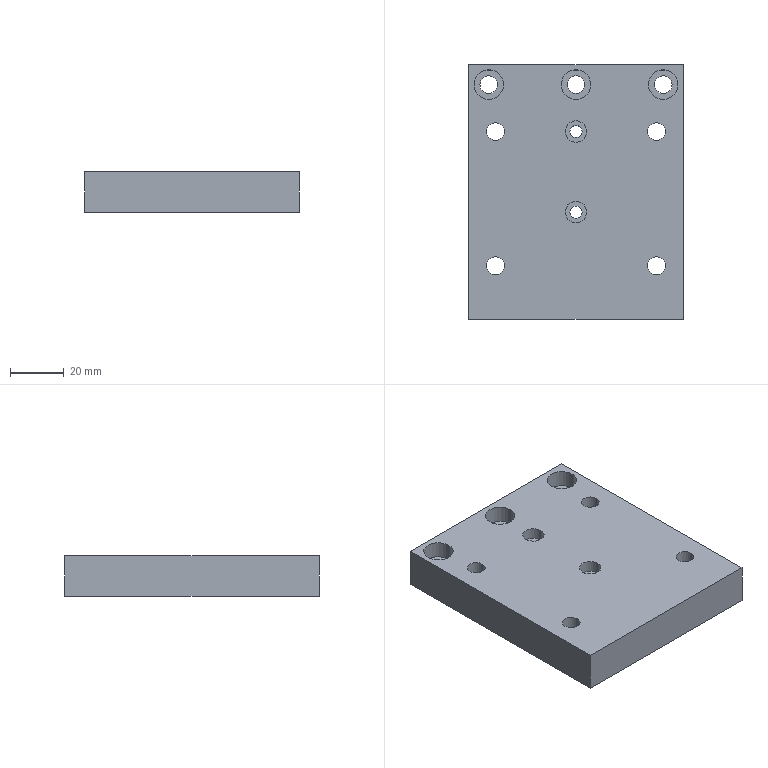Part | SolidWorks | features HoleWzd 3, Extrusion 1 | 1 solid | 51 faces | box 80 x 95 x 15 mm | volume 106903 mm3 | cylinder 36 | plane 15 | commonest cylinder face diameters 6.6 x14 11 x14 4.5 x4 8 x4
STEP:
#1=CARTESIAN_POINT('',(-38.,40.,8.6));
#2=VERTEX_POINT('',#1);
#3=CARTESIAN_POINT('',(-27.,40.,8.6));
#4=VERTEX_POINT('',#3);
#5=CARTESIAN_POINT('',(-32.5,40.,8.6));
#6=DIRECTION('',(0.,0.,1.));
#7=DIRECTION('',(1.,0.,0.));
#8=AXIS2_PLACEMENT_3D('',#5,#6,#7);
#9=CIRCLE('',#8,5.5);
#10=EDGE_CURVE('',#2,#4,#9,.T.);
#11=ORIENTED_EDGE('',*,*,#10,.F.);
#12=CARTESIAN_POINT('',(-38.,40.,15.));
#13=VERTEX_POINT('',#12);
#14=CARTESIAN_POINT('',(-38.,40.,15.));
#15=DIRECTION('',(0.,0.,1.));
#16=VECTOR('',#15,1000.);
#17=LINE('',#14,#16);
#18=EDGE_CURVE('',#2,#13,#17,.T.);
#19=ORIENTED_EDGE('',*,*,#18,.T.);
#20=CARTESIAN_POINT('',(-27.,40.,15.));
#21=VERTEX_POINT('',#20);
#22=CARTESIAN_POINT('',(-32.5,40.,15.));
#23=DIRECTION('',(0.,0.,1.));
#24=DIRECTION('',(1.,0.,0.));
#25=AXIS2_PLACEMENT_3D('',#22,#23,#24);
#26=CIRCLE('',#25,5.5);
#27=EDGE_CURVE('',#13,#21,#26,.T.);
#28=ORIENTED_EDGE('',*,*,#27,.T.);
#29=CARTESIAN_POINT('',(-27.,40.,15.));
#30=DIRECTION('',(0.,0.,1.));
#31=VECTOR('',#30,1000.);
#32=LINE('',#29,#31);
#33=EDGE_CURVE('',#4,#21,#32,.T.);
#34=ORIENTED_EDGE('',*,*,#33,.F.);
#35=EDGE_LOOP('',(#11,#19,#28,#34));
#36=FACE_OUTER_BOUND('',#35,.T.);
#37=CARTESIAN_POINT('',(-32.5,40.,15.));
#38=DIRECTION('',(0.,0.,1.));
#39=DIRECTION('',(1.,0.,0.));
#40=AXIS2_PLACEMENT_3D('',#37,#38,#39);
#41=CYLINDRICAL_SURFACE('',#40,5.5);
#42=ADVANCED_FACE('',(#36),#41,.F.);
#43=CARTESIAN_POINT('',(-35.8,40.,0.));
#44=VERTEX_POINT('',#43);
#45=CARTESIAN_POINT('',(-29.2,40.,0.));
#46=VERTEX_POINT('',#45);
#47=CARTESIAN_POINT('',(-32.5,40.,0.));
#48=DIRECTION('',(0.,0.,1.));
#49=DIRECTION('',(1.,0.,0.));
#50=AXIS2_PLACEMENT_3D('',#47,#48,#49);
#51=CIRCLE('',#50,3.3);
#52=EDGE_CURVE('',#44,#46,#51,.T.);
#53=ORIENTED_EDGE('',*,*,#52,.F.);
#54=CARTESIAN_POINT('',(-35.8,40.,8.6));
#55=VERTEX_POINT('',#54);
#56=CARTESIAN_POINT('',(-35.8,40.,15.));
#57=DIRECTION('',(0.,0.,1.));
#58=VECTOR('',#57,1000.);
#59=LINE('',#56,#58);
#60=EDGE_CURVE('',#44,#55,#59,.T.);
#61=ORIENTED_EDGE('',*,*,#60,.T.);
#62=CARTESIAN_POINT('',(-29.2,40.,8.6));
#63=VERTEX_POINT('',#62);
#64=CARTESIAN_POINT('',(-32.5,40.,8.6));
#65=DIRECTION('',(0.,0.,1.));
#66=DIRECTION('',(1.,0.,0.));
#67=AXIS2_PLACEMENT_3D('',#64,#65,#66);
#68=CIRCLE('',#67,3.3);
#69=EDGE_CURVE('',#55,#63,#68,.T.);
#70=ORIENTED_EDGE('',*,*,#69,.T.);
#71=CARTESIAN_POINT('',(-29.2,40.,15.));
#72=DIRECTION('',(0.,0.,1.));
#73=VECTOR('',#72,1000.);
#74=LINE('',#71,#73);
#75=EDGE_CURVE('',#46,#63,#74,.T.);
#76=ORIENTED_EDGE('',*,*,#75,.F.);
#77=EDGE_LOOP('',(#53,#61,#70,#76));
#78=FACE_OUTER_BOUND('',#77,.T.);
#79=CARTESIAN_POINT('',(-32.5,40.,15.));
#80=DIRECTION('',(0.,0.,1.));
#81=DIRECTION('',(1.,0.,0.));
#82=AXIS2_PLACEMENT_3D('',#79,#80,#81);
#83=CYLINDRICAL_SURFACE('',#82,3.3);
#84=ADVANCED_FACE('',(#78),#83,.F.);
#85=CARTESIAN_POINT('',(-5.5,40.,8.6));
#86=VERTEX_POINT('',#85);
#87=CARTESIAN_POINT('',(5.5,40.,8.6));
#88=VERTEX_POINT('',#87);
#89=CARTESIAN_POINT('',(0.,40.,8.6));
#90=DIRECTION('',(0.,0.,1.));
#91=DIRECTION('',(1.,0.,0.));
#92=AXIS2_PLACEMENT_3D('',#89,#90,#91);
#93=CIRCLE('',#92,5.5);
#94=EDGE_CURVE('',#86,#88,#93,.T.);
#95=ORIENTED_EDGE('',*,*,#94,.F.);
#96=CARTESIAN_POINT('',(-5.5,40.,15.));
#97=VERTEX_POINT('',#96);
#98=CARTESIAN_POINT('',(-5.5,40.,15.));
#99=DIRECTION('',(0.,0.,1.));
#100=VECTOR('',#99,1000.);
#101=LINE('',#98,#100);
#102=EDGE_CURVE('',#86,#97,#101,.T.);
#103=ORIENTED_EDGE('',*,*,#102,.T.);
#104=CARTESIAN_POINT('',(5.5,40.,15.));
#105=VERTEX_POINT('',#104);
#106=CARTESIAN_POINT('',(0.,40.,15.));
#107=DIRECTION('',(0.,0.,1.));
#108=DIRECTION('',(1.,0.,0.));
#109=AXIS2_PLACEMENT_3D('',#106,#107,#108);
#110=CIRCLE('',#109,5.5);
#111=EDGE_CURVE('',#97,#105,#110,.T.);
#112=ORIENTED_EDGE('',*,*,#111,.T.);
#113=CARTESIAN_POINT('',(5.5,40.,15.));
#114=DIRECTION('',(0.,0.,1.));
#115=VECTOR('',#114,1000.);
#116=LINE('',#113,#115);
#117=EDGE_CURVE('',#88,#105,#116,.T.);
#118=ORIENTED_EDGE('',*,*,#117,.F.);
#119=EDGE_LOOP('',(#95,#103,#112,#118));
#120=FACE_OUTER_BOUND('',#119,.T.);
#121=CARTESIAN_POINT('',(0.,40.,15.));
#122=DIRECTION('',(0.,0.,1.));
#123=DIRECTION('',(1.,0.,0.));
#124=AXIS2_PLACEMENT_3D('',#121,#122,#123);
#125=CYLINDRICAL_SURFACE('',#124,5.5);
#126=ADVANCED_FACE('',(#120),#125,.F.);
#127=CARTESIAN_POINT('',(-3.3,40.,0.));
#128=VERTEX_POINT('',#127);
#129=CARTESIAN_POINT('',(3.3,40.,0.));
#130=VERTEX_POINT('',#129);
#131=CARTESIAN_POINT('',(0.,40.,0.));
#132=DIRECTION('',(0.,0.,1.));
#133=DIRECTION('',(1.,0.,0.));
#134=AXIS2_PLACEMENT_3D('',#131,#132,#133);
#135=CIRCLE('',#134,3.3);
#136=EDGE_CURVE('',#128,#130,#135,.T.);
#137=ORIENTED_EDGE('',*,*,#136,.F.);
#138=CARTESIAN_POINT('',(-3.3,40.,8.6));
#139=VERTEX_POINT('',#138);
#140=CARTESIAN_POINT('',(-3.3,40.,15.));
#141=DIRECTION('',(0.,0.,1.));
#142=VECTOR('',#141,1000.);
#143=LINE('',#140,#142);
#144=EDGE_CURVE('',#128,#139,#143,.T.);
#145=ORIENTED_EDGE('',*,*,#144,.T.);
#146=CARTESIAN_POINT('',(3.3,40.,8.6));
#147=VERTEX_POINT('',#146);
#148=CARTESIAN_POINT('',(0.,40.,8.6));
#149=DIRECTION('',(0.,0.,1.));
#150=DIRECTION('',(1.,0.,0.));
#151=AXIS2_PLACEMENT_3D('',#148,#149,#150);
#152=CIRCLE('',#151,3.3);
#153=EDGE_CURVE('',#139,#147,#152,.T.);
#154=ORIENTED_EDGE('',*,*,#153,.T.);
#155=CARTESIAN_POINT('',(3.3,40.,15.));
#156=DIRECTION('',(0.,0.,1.));
#157=VECTOR('',#156,1000.);
#158=LINE('',#155,#157);
#159=EDGE_CURVE('',#130,#147,#158,.T.);
#160=ORIENTED_EDGE('',*,*,#159,.F.);
#161=EDGE_LOOP('',(#137,#145,#154,#160));
#162=FACE_OUTER_BOUND('',#161,.T.);
#163=CARTESIAN_POINT('',(0.,40.,15.));
#164=DIRECTION('',(0.,0.,1.));
#165=DIRECTION('',(1.,0.,0.));
#166=AXIS2_PLACEMENT_3D('',#163,#164,#165);
#167=CYLINDRICAL_SURFACE('',#166,3.3);
#168=ADVANCED_FACE('',(#162),#167,.F.);
#169=CARTESIAN_POINT('',(27.,40.,8.6));
#170=VERTEX_POINT('',#169);
#171=CARTESIAN_POINT('',(38.,40.,8.6));
#172=VERTEX_POINT('',#171);
#173=CARTESIAN_POINT('',(32.5,40.,8.6));
#174=DIRECTION('',(0.,0.,1.));
#175=DIRECTION('',(1.,0.,0.));
#176=AXIS2_PLACEMENT_3D('',#173,#174,#175);
#177=CIRCLE('',#176,5.5);
#178=EDGE_CURVE('',#170,#172,#177,.T.);
#179=ORIENTED_EDGE('',*,*,#178,.F.);
#180=CARTESIAN_POINT('',(27.,40.,15.));
#181=VERTEX_POINT('',#180);
#182=CARTESIAN_POINT('',(27.,40.,15.));
#183=DIRECTION('',(0.,0.,1.));
#184=VECTOR('',#183,1000.);
#185=LINE('',#182,#184);
#186=EDGE_CURVE('',#170,#181,#185,.T.);
#187=ORIENTED_EDGE('',*,*,#186,.T.);
#188=CARTESIAN_POINT('',(38.,40.,15.));
#189=VERTEX_POINT('',#188);
#190=CARTESIAN_POINT('',(32.5,40.,15.));
#191=DIRECTION('',(0.,0.,1.));
#192=DIRECTION('',(1.,0.,0.));
#193=AXIS2_PLACEMENT_3D('',#190,#191,#192);
#194=CIRCLE('',#193,5.5);
#195=EDGE_CURVE('',#181,#189,#194,.T.);
#196=ORIENTED_EDGE('',*,*,#195,.T.);
#197=CARTESIAN_POINT('',(38.,40.,15.));
#198=DIRECTION('',(0.,0.,1.));
#199=VECTOR('',#198,1000.);
#200=LINE('',#197,#199);
#201=EDGE_CURVE('',#172,#189,#200,.T.);
#202=ORIENTED_EDGE('',*,*,#201,.F.);
#203=EDGE_LOOP('',(#179,#187,#196,#202));
#204=FACE_OUTER_BOUND('',#203,.T.);
#205=CARTESIAN_POINT('',(32.5,40.,15.));
#206=DIRECTION('',(0.,0.,1.));
#207=DIRECTION('',(1.,0.,0.));
#208=AXIS2_PLACEMENT_3D('',#205,#206,#207);
#209=CYLINDRICAL_SURFACE('',#208,5.5);
#210=ADVANCED_FACE('',(#204),#209,.F.);
#211=CARTESIAN_POINT('',(29.2,40.,0.));
#212=VERTEX_POINT('',#211);
#213=CARTESIAN_POINT('',(35.8,40.,0.));
#214=VERTEX_POINT('',#213);
#215=CARTESIAN_POINT('',(32.5,40.,0.));
#216=DIRECTION('',(0.,0.,1.));
#217=DIRECTION('',(1.,0.,0.));
#218=AXIS2_PLACEMENT_3D('',#215,#216,#217);
#219=CIRCLE('',#218,3.3);
#220=EDGE_CURVE('',#212,#214,#219,.T.);
#221=ORIENTED_EDGE('',*,*,#220,.F.);
#222=CARTESIAN_POINT('',(29.2,40.,8.6));
#223=VERTEX_POINT('',#222);
#224=CARTESIAN_POINT('',(29.2,40.,15.));
#225=DIRECTION('',(0.,0.,1.));
#226=VECTOR('',#225,1000.);
#227=LINE('',#224,#226);
#228=EDGE_CURVE('',#212,#223,#227,.T.);
#229=ORIENTED_EDGE('',*,*,#228,.T.);
#230=CARTESIAN_POINT('',(35.8,40.,8.6));
#231=VERTEX_POINT('',#230);
#232=CARTESIAN_POINT('',(32.5,40.,8.6));
#233=DIRECTION('',(0.,0.,1.));
#234=DIRECTION('',(1.,0.,0.));
#235=AXIS2_PLACEMENT_3D('',#232,#233,#234);
#236=CIRCLE('',#235,3.3);
#237=EDGE_CURVE('',#223,#231,#236,.T.);
#238=ORIENTED_EDGE('',*,*,#237,.T.);
#239=CARTESIAN_POINT('',(35.8,40.,15.));
#240=DIRECTION('',(0.,0.,1.));
#241=VECTOR('',#240,1000.);
#242=LINE('',#239,#241);
#243=EDGE_CURVE('',#214,#231,#242,.T.);
#244=ORIENTED_EDGE('',*,*,#243,.F.);
#245=EDGE_LOOP('',(#221,#229,#238,#244));
#246=FACE_OUTER_BOUND('',#245,.T.);
#247=CARTESIAN_POINT('',(32.5,40.,15.));
#248=DIRECTION('',(0.,0.,1.));
#249=DIRECTION('',(1.,0.,0.));
#250=AXIS2_PLACEMENT_3D('',#247,#248,#249);
#251=CYLINDRICAL_SURFACE('',#250,3.3);
#252=ADVANCED_FACE('',(#246),#251,.F.);
#253=CARTESIAN_POINT('',(35.5,22.5,6.4));
#254=VERTEX_POINT('',#253);
#255=CARTESIAN_POINT('',(24.5,22.5,6.4));
#256=VERTEX_POINT('',#255);
#257=CARTESIAN_POINT('',(30.,22.5,6.4));
#258=DIRECTION('',(0.,0.,-1.));
#259=DIRECTION('',(-1.,0.,0.));
#260=AXIS2_PLACEMENT_3D('',#257,#258,#259);
#261=CIRCLE('',#260,5.5);
#262=EDGE_CURVE('',#254,#256,#261,.T.);
#263=ORIENTED_EDGE('',*,*,#262,.F.);
#264=CARTESIAN_POINT('',(35.5,22.5,0.));
#265=VERTEX_POINT('',#264);
#266=CARTESIAN_POINT('',(35.5,22.5,0.));
#267=DIRECTION('',(0.,0.,-1.));
#268=VECTOR('',#267,1000.);
#269=LINE('',#266,#268);
#270=EDGE_CURVE('',#254,#265,#269,.T.);
#271=ORIENTED_EDGE('',*,*,#270,.T.);
#272=CARTESIAN_POINT('',(24.5,22.5,0.));
#273=VERTEX_POINT('',#272);
#274=CARTESIAN_POINT('',(30.,22.5,0.));
#275=DIRECTION('',(0.,0.,-1.));
#276=DIRECTION('',(-1.,0.,0.));
#277=AXIS2_PLACEMENT_3D('',#274,#275,#276);
#278=CIRCLE('',#277,5.5);
#279=EDGE_CURVE('',#265,#273,#278,.T.);
#280=ORIENTED_EDGE('',*,*,#279,.T.);
#281=CARTESIAN_POINT('',(24.5,22.5,0.));
#282=DIRECTION('',(0.,0.,-1.));
#283=VECTOR('',#282,1000.);
#284=LINE('',#281,#283);
#285=EDGE_CURVE('',#256,#273,#284,.T.);
#286=ORIENTED_EDGE('',*,*,#285,.F.);
#287=EDGE_LOOP('',(#263,#271,#280,#286));
#288=FACE_OUTER_BOUND('',#287,.T.);
#289=CARTESIAN_POINT('',(30.,22.5,0.));
#290=DIRECTION('',(0.,0.,-1.));
#291=DIRECTION('',(-1.,0.,0.));
#292=AXIS2_PLACEMENT_3D('',#289,#290,#291);
#293=CYLINDRICAL_SURFACE('',#292,5.5);
#294=ADVANCED_FACE('',(#288),#293,.F.);
#295=CARTESIAN_POINT('',(33.3,22.5,15.));
#296=VERTEX_POINT('',#295);
#297=CARTESIAN_POINT('',(26.7,22.5,15.));
#298=VERTEX_POINT('',#297);
#299=CARTESIAN_POINT('',(30.,22.5,15.));
#300=DIRECTION('',(0.,0.,-1.));
#301=DIRECTION('',(-1.,0.,0.));
#302=AXIS2_PLACEMENT_3D('',#299,#300,#301);
#303=CIRCLE('',#302,3.3);
#304=EDGE_CURVE('',#296,#298,#303,.T.);
#305=ORIENTED_EDGE('',*,*,#304,.F.);
#306=CARTESIAN_POINT('',(33.3,22.5,6.4));
#307=VERTEX_POINT('',#306);
#308=CARTESIAN_POINT('',(33.3,22.5,0.));
#309=DIRECTION('',(0.,0.,-1.));
#310=VECTOR('',#309,1000.);
#311=LINE('',#308,#310);
#312=EDGE_CURVE('',#296,#307,#311,.T.);
#313=ORIENTED_EDGE('',*,*,#312,.T.);
#314=CARTESIAN_POINT('',(26.7,22.5,6.4));
#315=VERTEX_POINT('',#314);
#316=CARTESIAN_POINT('',(30.,22.5,6.4));
#317=DIRECTION('',(0.,0.,-1.));
#318=DIRECTION('',(-1.,0.,0.));
#319=AXIS2_PLACEMENT_3D('',#316,#317,#318);
#320=CIRCLE('',#319,3.3);
#321=EDGE_CURVE('',#307,#315,#320,.T.);
#322=ORIENTED_EDGE('',*,*,#321,.T.);
#323=CARTESIAN_POINT('',(26.7,22.5,0.));
#324=DIRECTION('',(0.,0.,-1.));
#325=VECTOR('',#324,1000.);
#326=LINE('',#323,#325);
#327=EDGE_CURVE('',#298,#315,#326,.T.);
#328=ORIENTED_EDGE('',*,*,#327,.F.);
#329=EDGE_LOOP('',(#305,#313,#322,#328));
#330=FACE_OUTER_BOUND('',#329,.T.);
#331=CARTESIAN_POINT('',(30.,22.5,0.));
#332=DIRECTION('',(0.,0.,-1.));
#333=DIRECTION('',(-1.,0.,0.));
#334=AXIS2_PLACEMENT_3D('',#331,#332,#333);
#335=CYLINDRICAL_SURFACE('',#334,3.3);
#336=ADVANCED_FACE('',(#330),#335,.F.);
#337=CARTESIAN_POINT('',(-24.5,22.5,6.4));
#338=VERTEX_POINT('',#337);
#339=CARTESIAN_POINT('',(-35.5,22.5,6.4));
#340=VERTEX_POINT('',#339);
#341=CARTESIAN_POINT('',(-30.,22.5,6.4));
#342=DIRECTION('',(0.,0.,-1.));
#343=DIRECTION('',(-1.,0.,0.));
#344=AXIS2_PLACEMENT_3D('',#341,#342,#343);
#345=CIRCLE('',#344,5.5);
#346=EDGE_CURVE('',#338,#340,#345,.T.);
#347=ORIENTED_EDGE('',*,*,#346,.F.);
#348=CARTESIAN_POINT('',(-24.5,22.5,0.));
#349=VERTEX_POINT('',#348);
#350=CARTESIAN_POINT('',(-24.5,22.5,0.));
#351=DIRECTION('',(0.,0.,-1.));
#352=VECTOR('',#351,1000.);
#353=LINE('',#350,#352);
#354=EDGE_CURVE('',#338,#349,#353,.T.);
#355=ORIENTED_EDGE('',*,*,#354,.T.);
#356=CARTESIAN_POINT('',(-35.5,22.5,0.));
#357=VERTEX_POINT('',#356);
#358=CARTESIAN_POINT('',(-30.,22.5,0.));
#359=DIRECTION('',(0.,0.,-1.));
#360=DIRECTION('',(-1.,0.,0.));
#361=AXIS2_PLACEMENT_3D('',#358,#359,#360);
#362=CIRCLE('',#361,5.5);
#363=EDGE_CURVE('',#349,#357,#362,.T.);
#364=ORIENTED_EDGE('',*,*,#363,.T.);
#365=CARTESIAN_POINT('',(-35.5,22.5,0.));
#366=DIRECTION('',(0.,0.,-1.));
#367=VECTOR('',#366,1000.);
#368=LINE('',#365,#367);
#369=EDGE_CURVE('',#340,#357,#368,.T.);
#370=ORIENTED_EDGE('',*,*,#369,.F.);
#371=EDGE_LOOP('',(#347,#355,#364,#370));
#372=FACE_OUTER_BOUND('',#371,.T.);
#373=CARTESIAN_POINT('',(-30.,22.5,0.));
#374=DIRECTION('',(0.,0.,-1.));
#375=DIRECTION('',(-1.,0.,0.));
#376=AXIS2_PLACEMENT_3D('',#373,#374,#375);
#377=CYLINDRICAL_SURFACE('',#376,5.5);
#378=ADVANCED_FACE('',(#372),#377,.F.);
#379=CARTESIAN_POINT('',(-26.7,22.5,15.));
#380=VERTEX_POINT('',#379);
#381=CARTESIAN_POINT('',(-33.3,22.5,15.));
#382=VERTEX_POINT('',#381);
#383=CARTESIAN_POINT('',(-30.,22.5,15.));
#384=DIRECTION('',(0.,0.,-1.));
#385=DIRECTION('',(-1.,0.,0.));
#386=AXIS2_PLACEMENT_3D('',#383,#384,#385);
#387=CIRCLE('',#386,3.3);
#388=EDGE_CURVE('',#380,#382,#387,.T.);
#389=ORIENTED_EDGE('',*,*,#388,.F.);
#390=CARTESIAN_POINT('',(-26.7,22.5,6.4));
#391=VERTEX_POINT('',#390);
#392=CARTESIAN_POINT('',(-26.7,22.5,0.));
#393=DIRECTION('',(0.,0.,-1.));
#394=VECTOR('',#393,1000.);
#395=LINE('',#392,#394);
#396=EDGE_CURVE('',#380,#391,#395,.T.);
#397=ORIENTED_EDGE('',*,*,#396,.T.);
#398=CARTESIAN_POINT('',(-33.3,22.5,6.4));
#399=VERTEX_POINT('',#398);
#400=CARTESIAN_POINT('',(-30.,22.5,6.4));
#401=DIRECTION('',(0.,0.,-1.));
#402=DIRECTION('',(-1.,0.,0.));
#403=AXIS2_PLACEMENT_3D('',#400,#401,#402);
#404=CIRCLE('',#403,3.3);
#405=EDGE_CURVE('',#391,#399,#404,.T.);
#406=ORIENTED_EDGE('',*,*,#405,.T.);
#407=CARTESIAN_POINT('',(-33.3,22.5,0.));
#408=DIRECTION('',(0.,0.,-1.));
#409=VECTOR('',#408,1000.);
#410=LINE('',#407,#409);
#411=EDGE_CURVE('',#382,#399,#410,.T.);
#412=ORIENTED_EDGE('',*,*,#411,.F.);
#413=EDGE_LOOP('',(#389,#397,#406,#412));
#414=FACE_OUTER_BOUND('',#413,.T.);
#415=CARTESIAN_POINT('',(-30.,22.5,0.));
#416=DIRECTION('',(0.,0.,-1.));
#417=DIRECTION('',(-1.,0.,0.));
#418=AXIS2_PLACEMENT_3D('',#415,#416,#417);
#419=CYLINDRICAL_SURFACE('',#418,3.3);
#420=ADVANCED_FACE('',(#414),#419,.F.);
#421=CARTESIAN_POINT('',(-24.5,-27.5,6.4));
#422=VERTEX_POINT('',#421);
#423=CARTESIAN_POINT('',(-35.5,-27.5,6.4));
#424=VERTEX_POINT('',#423);
#425=CARTESIAN_POINT('',(-30.,-27.5,6.4));
#426=DIRECTION('',(0.,0.,-1.));
#427=DIRECTION('',(-1.,0.,0.));
#428=AXIS2_PLACEMENT_3D('',#425,#426,#427);
#429=CIRCLE('',#428,5.5);
#430=EDGE_CURVE('',#422,#424,#429,.T.);
#431=ORIENTED_EDGE('',*,*,#430,.F.);
#432=CARTESIAN_POINT('',(-24.5,-27.5,0.));
#433=VERTEX_POINT('',#432);
#434=CARTESIAN_POINT('',(-24.5,-27.5,0.));
#435=DIRECTION('',(0.,0.,-1.));
#436=VECTOR('',#435,1000.);
#437=LINE('',#434,#436);
#438=EDGE_CURVE('',#422,#433,#437,.T.);
#439=ORIENTED_EDGE('',*,*,#438,.T.);
#440=CARTESIAN_POINT('',(-35.5,-27.5,0.));
#441=VERTEX_POINT('',#440);
#442=CARTESIAN_POINT('',(-30.,-27.5,0.));
#443=DIRECTION('',(0.,0.,-1.));
#444=DIRECTION('',(-1.,0.,0.));
#445=AXIS2_PLACEMENT_3D('',#442,#443,#444);
#446=CIRCLE('',#445,5.5);
#447=EDGE_CURVE('',#433,#441,#446,.T.);
#448=ORIENTED_EDGE('',*,*,#447,.T.);
#449=CARTESIAN_POINT('',(-35.5,-27.5,0.));
#450=DIRECTION('',(0.,0.,-1.));
#451=VECTOR('',#450,1000.);
#452=LINE('',#449,#451);
#453=EDGE_CURVE('',#424,#441,#452,.T.);
#454=ORIENTED_EDGE('',*,*,#453,.F.);
#455=EDGE_LOOP('',(#431,#439,#448,#454));
#456=FACE_OUTER_BOUND('',#455,.T.);
#457=CARTESIAN_POINT('',(-30.,-27.5,0.));
#458=DIRECTION('',(0.,0.,-1.));
#459=DIRECTION('',(-1.,0.,0.));
#460=AXIS2_PLACEMENT_3D('',#457,#458,#459);
#461=CYLINDRICAL_SURFACE('',#460,5.5);
#462=ADVANCED_FACE('',(#456),#461,.F.);
#463=CARTESIAN_POINT('',(-26.7,-27.5,15.));
#464=VERTEX_POINT('',#463);
#465=CARTESIAN_POINT('',(-33.3,-27.5,15.));
#466=VERTEX_POINT('',#465);
#467=CARTESIAN_POINT('',(-30.,-27.5,15.));
#468=DIRECTION('',(0.,0.,-1.));
#469=DIRECTION('',(-1.,0.,0.));
#470=AXIS2_PLACEMENT_3D('',#467,#468,#469);
#471=CIRCLE('',#470,3.3);
#472=EDGE_CURVE('',#464,#466,#471,.T.);
#473=ORIENTED_EDGE('',*,*,#472,.F.);
#474=CARTESIAN_POINT('',(-26.7,-27.5,6.4));
#475=VERTEX_POINT('',#474);
#476=CARTESIAN_POINT('',(-26.7,-27.5,0.));
#477=DIRECTION('',(0.,0.,-1.));
#478=VECTOR('',#477,1000.);
#479=LINE('',#476,#478);
#480=EDGE_CURVE('',#464,#475,#479,.T.);
#481=ORIENTED_EDGE('',*,*,#480,.T.);
#482=CARTESIAN_POINT('',(-33.3,-27.5,6.4));
#483=VERTEX_POINT('',#482);
#484=CARTESIAN_POINT('',(-30.,-27.5,6.4));
#485=DIRECTION('',(0.,0.,-1.));
#486=DIRECTION('',(-1.,0.,0.));
#487=AXIS2_PLACEMENT_3D('',#484,#485,#486);
#488=CIRCLE('',#487,3.3);
#489=EDGE_CURVE('',#475,#483,#488,.T.);
#490=ORIENTED_EDGE('',*,*,#489,.T.);
#491=CARTESIAN_POINT('',(-33.3,-27.5,0.));
#492=DIRECTION('',(0.,0.,-1.));
#493=VECTOR('',#492,1000.);
#494=LINE('',#491,#493);
#495=EDGE_CURVE('',#466,#483,#494,.T.);
#496=ORIENTED_EDGE('',*,*,#495,.F.);
#497=EDGE_LOOP('',(#473,#481,#490,#496));
#498=FACE_OUTER_BOUND('',#497,.T.);
#499=CARTESIAN_POINT('',(-30.,-27.5,0.));
#500=DIRECTION('',(0.,0.,-1.));
#501=DIRECTION('',(-1.,0.,0.));
#502=AXIS2_PLACEMENT_3D('',#499,#500,#501);
#503=CYLINDRICAL_SURFACE('',#502,3.3);
#504=ADVANCED_FACE('',(#498),#503,.F.);
#505=CARTESIAN_POINT('',(35.5,-27.5,6.4));
#506=VERTEX_POINT('',#505);
#507=CARTESIAN_POINT('',(24.5,-27.5,6.4));
#508=VERTEX_POINT('',#507);
#509=CARTESIAN_POINT('',(30.,-27.5,6.4));
#510=DIRECTION('',(0.,0.,-1.));
#511=DIRECTION('',(-1.,0.,0.));
#512=AXIS2_PLACEMENT_3D('',#509,#510,#511);
#513=CIRCLE('',#512,5.5);
#514=EDGE_CURVE('',#506,#508,#513,.T.);
#515=ORIENTED_EDGE('',*,*,#514,.F.);
#516=CARTESIAN_POINT('',(35.5,-27.5,0.));
#517=VERTEX_POINT('',#516);
#518=CARTESIAN_POINT('',(35.5,-27.5,0.));
#519=DIRECTION('',(0.,0.,-1.));
#520=VECTOR('',#519,1000.);
#521=LINE('',#518,#520);
#522=EDGE_CURVE('',#506,#517,#521,.T.);
#523=ORIENTED_EDGE('',*,*,#522,.T.);
#524=CARTESIAN_POINT('',(24.5,-27.5,0.));
#525=VERTEX_POINT('',#524);
#526=CARTESIAN_POINT('',(30.,-27.5,0.));
#527=DIRECTION('',(0.,0.,-1.));
#528=DIRECTION('',(-1.,0.,0.));
#529=AXIS2_PLACEMENT_3D('',#526,#527,#528);
#530=CIRCLE('',#529,5.5);
#531=EDGE_CURVE('',#517,#525,#530,.T.);
#532=ORIENTED_EDGE('',*,*,#531,.T.);
#533=CARTESIAN_POINT('',(24.5,-27.5,0.));
#534=DIRECTION('',(0.,0.,-1.));
#535=VECTOR('',#534,1000.);
#536=LINE('',#533,#535);
#537=EDGE_CURVE('',#508,#525,#536,.T.);
#538=ORIENTED_EDGE('',*,*,#537,.F.);
#539=EDGE_LOOP('',(#515,#523,#532,#538));
#540=FACE_OUTER_BOUND('',#539,.T.);
#541=CARTESIAN_POINT('',(30.,-27.5,0.));
#542=DIRECTION('',(0.,0.,-1.));
#543=DIRECTION('',(-1.,0.,0.));
#544=AXIS2_PLACEMENT_3D('',#541,#542,#543);
#545=CYLINDRICAL_SURFACE('',#544,5.5);
#546=ADVANCED_FACE('',(#540),#545,.F.);
#547=CARTESIAN_POINT('',(33.3,-27.5,15.));
#548=VERTEX_POINT('',#547);
#549=CARTESIAN_POINT('',(26.7,-27.5,15.));
#550=VERTEX_POINT('',#549);
#551=CARTESIAN_POINT('',(30.,-27.5,15.));
#552=DIRECTION('',(0.,0.,-1.));
#553=DIRECTION('',(-1.,0.,0.));
#554=AXIS2_PLACEMENT_3D('',#551,#552,#553);
#555=CIRCLE('',#554,3.3);
#556=EDGE_CURVE('',#548,#550,#555,.T.);
#557=ORIENTED_EDGE('',*,*,#556,.F.);
#558=CARTESIAN_POINT('',(33.3,-27.5,6.4));
#559=VERTEX_POINT('',#558);
#560=CARTESIAN_POINT('',(33.3,-27.5,0.));
#561=DIRECTION('',(0.,0.,-1.));
#562=VECTOR('',#561,1000.);
#563=LINE('',#560,#562);
#564=EDGE_CURVE('',#548,#559,#563,.T.);
#565=ORIENTED_EDGE('',*,*,#564,.T.);
#566=CARTESIAN_POINT('',(26.7,-27.5,6.4));
#567=VERTEX_POINT('',#566);
#568=CARTESIAN_POINT('',(30.,-27.5,6.4));
#569=DIRECTION('',(0.,0.,-1.));
#570=DIRECTION('',(-1.,0.,0.));
#571=AXIS2_PLACEMENT_3D('',#568,#569,#570);
#572=CIRCLE('',#571,3.3);
#573=EDGE_CURVE('',#559,#567,#572,.T.);
#574=ORIENTED_EDGE('',*,*,#573,.T.);
#575=CARTESIAN_POINT('',(26.7,-27.5,0.));
#576=DIRECTION('',(0.,0.,-1.));
#577=VECTOR('',#576,1000.);
#578=LINE('',#575,#577);
#579=EDGE_CURVE('',#550,#567,#578,.T.);
#580=ORIENTED_EDGE('',*,*,#579,.F.);
#581=EDGE_LOOP('',(#557,#565,#574,#580));
#582=FACE_OUTER_BOUND('',#581,.T.);
#583=CARTESIAN_POINT('',(30.,-27.5,0.));
#584=DIRECTION('',(0.,0.,-1.));
#585=DIRECTION('',(-1.,0.,0.));
#586=AXIS2_PLACEMENT_3D('',#583,#584,#585);
#587=CYLINDRICAL_SURFACE('',#586,3.3);
#588=ADVANCED_FACE('',(#582),#587,.F.);
#589=CARTESIAN_POINT('',(-4.,22.5,10.6));
#590=VERTEX_POINT('',#589);
#591=CARTESIAN_POINT('',(4.,22.5,10.6));
#592=VERTEX_POINT('',#591);
#593=CARTESIAN_POINT('',(0.,22.5,10.6));
#594=DIRECTION('',(0.,0.,1.));
#595=DIRECTION('',(1.,0.,0.));
#596=AXIS2_PLACEMENT_3D('',#593,#594,#595);
#597=CIRCLE('',#596,4.);
#598=EDGE_CURVE('',#590,#592,#597,.T.);
#599=ORIENTED_EDGE('',*,*,#598,.F.);
#600=CARTESIAN_POINT('',(-4.,22.5,15.));
#601=VERTEX_POINT('',#600);
#602=CARTESIAN_POINT('',(-4.,22.5,15.));
#603=DIRECTION('',(0.,0.,1.));
#604=VECTOR('',#603,1000.);
#605=LINE('',#602,#604);
#606=EDGE_CURVE('',#590,#601,#605,.T.);
#607=ORIENTED_EDGE('',*,*,#606,.T.);
#608=CARTESIAN_POINT('',(4.,22.5,15.));
#609=VERTEX_POINT('',#608);
#610=CARTESIAN_POINT('',(0.,22.5,15.));
#611=DIRECTION('',(0.,0.,1.));
#612=DIRECTION('',(1.,0.,0.));
#613=AXIS2_PLACEMENT_3D('',#610,#611,#612);
#614=CIRCLE('',#613,4.);
#615=EDGE_CURVE('',#601,#609,#614,.T.);
#616=ORIENTED_EDGE('',*,*,#615,.T.);
#617=CARTESIAN_POINT('',(4.,22.5,15.));
#618=DIRECTION('',(0.,0.,1.));
#619=VECTOR('',#618,1000.);
#620=LINE('',#617,#619);
#621=EDGE_CURVE('',#592,#609,#620,.T.);
#622=ORIENTED_EDGE('',*,*,#621,.F.);
#623=EDGE_LOOP('',(#599,#607,#616,#622));
#624=FACE_OUTER_BOUND('',#623,.T.);
#625=CARTESIAN_POINT('',(0.,22.5,15.));
#626=DIRECTION('',(0.,0.,1.));
#627=DIRECTION('',(1.,0.,0.));
#628=AXIS2_PLACEMENT_3D('',#625,#626,#627);
#629=CYLINDRICAL_SURFACE('',#628,4.);
#630=ADVANCED_FACE('',(#624),#629,.F.);
#631=CARTESIAN_POINT('',(-2.25,22.5,0.));
#632=VERTEX_POINT('',#631);
#633=CARTESIAN_POINT('',(2.25,22.5,0.));
#634=VERTEX_POINT('',#633);
#635=CARTESIAN_POINT('',(0.,22.5,0.));
#636=DIRECTION('',(0.,0.,1.));
#637=DIRECTION('',(1.,0.,0.));
#638=AXIS2_PLACEMENT_3D('',#635,#636,#637);
#639=CIRCLE('',#638,2.25);
#640=EDGE_CURVE('',#632,#634,#639,.T.);
#641=ORIENTED_EDGE('',*,*,#640,.F.);
#642=CARTESIAN_POINT('',(-2.25,22.5,10.6));
#643=VERTEX_POINT('',#642);
#644=CARTESIAN_POINT('',(-2.25,22.5,15.));
#645=DIRECTION('',(0.,0.,1.));
#646=VECTOR('',#645,1000.);
#647=LINE('',#644,#646);
#648=EDGE_CURVE('',#632,#643,#647,.T.);
#649=ORIENTED_EDGE('',*,*,#648,.T.);
#650=CARTESIAN_POINT('',(2.25,22.5,10.6));
#651=VERTEX_POINT('',#650);
#652=CARTESIAN_POINT('',(0.,22.5,10.6));
#653=DIRECTION('',(0.,0.,1.));
#654=DIRECTION('',(1.,0.,0.));
#655=AXIS2_PLACEMENT_3D('',#652,#653,#654);
#656=CIRCLE('',#655,2.25);
#657=EDGE_CURVE('',#643,#651,#656,.T.);
#658=ORIENTED_EDGE('',*,*,#657,.T.);
#659=CARTESIAN_POINT('',(2.25,22.5,15.));
#660=DIRECTION('',(0.,0.,1.));
#661=VECTOR('',#660,1000.);
#662=LINE('',#659,#661);
#663=EDGE_CURVE('',#634,#651,#662,.T.);
#664=ORIENTED_EDGE('',*,*,#663,.F.);
#665=EDGE_LOOP('',(#641,#649,#658,#664));
#666=FACE_OUTER_BOUND('',#665,.T.);
#667=CARTESIAN_POINT('',(0.,22.5,15.));
#668=DIRECTION('',(0.,0.,1.));
#669=DIRECTION('',(1.,0.,0.));
#670=AXIS2_PLACEMENT_3D('',#667,#668,#669);
#671=CYLINDRICAL_SURFACE('',#670,2.25);
#672=ADVANCED_FACE('',(#666),#671,.F.);
#673=CARTESIAN_POINT('',(-4.,-7.5,10.6));
#674=VERTEX_POINT('',#673);
#675=CARTESIAN_POINT('',(4.,-7.5,10.6));
#676=VERTEX_POINT('',#675);
#677=CARTESIAN_POINT('',(0.,-7.5,10.6));
#678=DIRECTION('',(0.,0.,1.));
#679=DIRECTION('',(1.,0.,0.));
#680=AXIS2_PLACEMENT_3D('',#677,#678,#679);
#681=CIRCLE('',#680,4.);
#682=EDGE_CURVE('',#674,#676,#681,.T.);
#683=ORIENTED_EDGE('',*,*,#682,.F.);
#684=CARTESIAN_POINT('',(-4.,-7.5,15.));
#685=VERTEX_POINT('',#684);
#686=CARTESIAN_POINT('',(-4.,-7.5,15.));
#687=DIRECTION('',(0.,0.,1.));
#688=VECTOR('',#687,1000.);
#689=LINE('',#686,#688);
#690=EDGE_CURVE('',#674,#685,#689,.T.);
#691=ORIENTED_EDGE('',*,*,#690,.T.);
#692=CARTESIAN_POINT('',(4.,-7.5,15.));
#693=VERTEX_POINT('',#692);
#694=CARTESIAN_POINT('',(0.,-7.5,15.));
#695=DIRECTION('',(0.,0.,1.));
#696=DIRECTION('',(1.,0.,0.));
#697=AXIS2_PLACEMENT_3D('',#694,#695,#696);
#698=CIRCLE('',#697,4.);
#699=EDGE_CURVE('',#685,#693,#698,.T.);
#700=ORIENTED_EDGE('',*,*,#699,.T.);
#701=CARTESIAN_POINT('',(4.,-7.5,15.));
#702=DIRECTION('',(0.,0.,1.));
#703=VECTOR('',#702,1000.);
#704=LINE('',#701,#703);
#705=EDGE_CURVE('',#676,#693,#704,.T.);
#706=ORIENTED_EDGE('',*,*,#705,.F.);
#707=EDGE_LOOP('',(#683,#691,#700,#706));
#708=FACE_OUTER_BOUND('',#707,.T.);
#709=CARTESIAN_POINT('',(0.,-7.5,15.));
#710=DIRECTION('',(0.,0.,1.));
#711=DIRECTION('',(1.,0.,0.));
#712=AXIS2_PLACEMENT_3D('',#709,#710,#711);
#713=CYLINDRICAL_SURFACE('',#712,4.);
#714=ADVANCED_FACE('',(#708),#713,.F.);
#715=CARTESIAN_POINT('',(-2.25,-7.5,0.));
#716=VERTEX_POINT('',#715);
#717=CARTESIAN_POINT('',(2.25,-7.5,0.));
#718=VERTEX_POINT('',#717);
#719=CARTESIAN_POINT('',(0.,-7.5,0.));
#720=DIRECTION('',(0.,0.,1.));
#721=DIRECTION('',(1.,0.,0.));
#722=AXIS2_PLACEMENT_3D('',#719,#720,#721);
#723=CIRCLE('',#722,2.25);
#724=EDGE_CURVE('',#716,#718,#723,.T.);
#725=ORIENTED_EDGE('',*,*,#724,.F.);
#726=CARTESIAN_POINT('',(-2.25,-7.5,10.6));
#727=VERTEX_POINT('',#726);
#728=CARTESIAN_POINT('',(-2.25,-7.5,15.));
#729=DIRECTION('',(0.,0.,1.));
#730=VECTOR('',#729,1000.);
#731=LINE('',#728,#730);
#732=EDGE_CURVE('',#716,#727,#731,.T.);
#733=ORIENTED_EDGE('',*,*,#732,.T.);
#734=CARTESIAN_POINT('',(2.25,-7.5,10.6));
#735=VERTEX_POINT('',#734);
#736=CARTESIAN_POINT('',(0.,-7.5,10.6));
#737=DIRECTION('',(0.,0.,1.));
#738=DIRECTION('',(1.,0.,0.));
#739=AXIS2_PLACEMENT_3D('',#736,#737,#738);
#740=CIRCLE('',#739,2.25);
#741=EDGE_CURVE('',#727,#735,#740,.T.);
#742=ORIENTED_EDGE('',*,*,#741,.T.);
#743=CARTESIAN_POINT('',(2.25,-7.5,15.));
#744=DIRECTION('',(0.,0.,1.));
#745=VECTOR('',#744,1000.);
#746=LINE('',#743,#745);
#747=EDGE_CURVE('',#718,#735,#746,.T.);
#748=ORIENTED_EDGE('',*,*,#747,.F.);
#749=EDGE_LOOP('',(#725,#733,#742,#748));
#750=FACE_OUTER_BOUND('',#749,.T.);
#751=CARTESIAN_POINT('',(0.,-7.5,15.));
#752=DIRECTION('',(0.,0.,1.));
#753=DIRECTION('',(1.,0.,0.));
#754=AXIS2_PLACEMENT_3D('',#751,#752,#753);
#755=CYLINDRICAL_SURFACE('',#754,2.25);
#756=ADVANCED_FACE('',(#750),#755,.F.);
#757=CARTESIAN_POINT('',(40.,-47.5,0.));
#758=VERTEX_POINT('',#757);
#759=CARTESIAN_POINT('',(40.,47.5,0.));
#760=VERTEX_POINT('',#759);
#761=CARTESIAN_POINT('',(40.,47.5,0.));
#762=DIRECTION('',(0.,1.,0.));
#763=VECTOR('',#762,1000.);
#764=LINE('',#761,#763);
#765=EDGE_CURVE('',#758,#760,#764,.T.);
#766=ORIENTED_EDGE('',*,*,#765,.T.);
#767=CARTESIAN_POINT('',(40.,47.5,15.));
#768=VERTEX_POINT('',#767);
#769=CARTESIAN_POINT('',(40.,47.5,15.));
#770=DIRECTION('',(0.,0.,-1.));
#771=VECTOR('',#770,1000.);
#772=LINE('',#769,#771);
#773=EDGE_CURVE('',#768,#760,#772,.T.);
#774=ORIENTED_EDGE('',*,*,#773,.F.);
#775=CARTESIAN_POINT('',(40.,-47.5,15.));
#776=VERTEX_POINT('',#775);
#777=CARTESIAN_POINT('',(40.,47.5,15.));
#778=DIRECTION('',(0.,1.,0.));
#779=VECTOR('',#778,1000.);
#780=LINE('',#777,#779);
#781=EDGE_CURVE('',#776,#768,#780,.T.);
#782=ORIENTED_EDGE('',*,*,#781,.F.);
#783=CARTESIAN_POINT('',(40.,-47.5,15.));
#784=DIRECTION('',(0.,0.,-1.));
#785=VECTOR('',#784,1000.);
#786=LINE('',#783,#785);
#787=EDGE_CURVE('',#776,#758,#786,.T.);
#788=ORIENTED_EDGE('',*,*,#787,.T.);
#789=EDGE_LOOP('',(#766,#774,#782,#788));
#790=FACE_OUTER_BOUND('',#789,.T.);
#791=CARTESIAN_POINT('',(40.,47.5,15.));
#792=DIRECTION('',(-1.,0.,0.));
#793=DIRECTION('',(0.,-1.,0.));
#794=AXIS2_PLACEMENT_3D('',#791,#792,#793);
#795=PLANE('',#794);
#796=ADVANCED_FACE('',(#790),#795,.F.);
#797=CARTESIAN_POINT('',(-40.,47.5,0.));
#798=VERTEX_POINT('',#797);
#799=CARTESIAN_POINT('',(-40.,47.5,0.));
#800=DIRECTION('',(-1.,0.,0.));
#801=VECTOR('',#800,1000.);
#802=LINE('',#799,#801);
#803=EDGE_CURVE('',#760,#798,#802,.T.);
#804=ORIENTED_EDGE('',*,*,#803,.T.);
#805=CARTESIAN_POINT('',(-40.,47.5,15.));
#806=VERTEX_POINT('',#805);
#807=CARTESIAN_POINT('',(-40.,47.5,15.));
#808=DIRECTION('',(0.,0.,-1.));
#809=VECTOR('',#808,1000.);
#810=LINE('',#807,#809);
#811=EDGE_CURVE('',#806,#798,#810,.T.);
#812=ORIENTED_EDGE('',*,*,#811,.F.);
#813=CARTESIAN_POINT('',(-40.,47.5,15.));
#814=DIRECTION('',(-1.,0.,0.));
#815=VECTOR('',#814,1000.);
#816=LINE('',#813,#815);
#817=EDGE_CURVE('',#768,#806,#816,.T.);
#818=ORIENTED_EDGE('',*,*,#817,.F.);
#819=ORIENTED_EDGE('',*,*,#773,.T.);
#820=EDGE_LOOP('',(#804,#812,#818,#819));
#821=FACE_OUTER_BOUND('',#820,.T.);
#822=CARTESIAN_POINT('',(-40.,47.5,15.));
#823=DIRECTION('',(0.,-1.,0.));
#824=DIRECTION('',(0.,0.,-1.));
#825=AXIS2_PLACEMENT_3D('',#822,#823,#824);
#826=PLANE('',#825);
#827=ADVANCED_FACE('',(#821),#826,.F.);
#828=CARTESIAN_POINT('',(-40.,-47.5,0.));
#829=VERTEX_POINT('',#828);
#830=CARTESIAN_POINT('',(-40.,47.5,0.));
#831=DIRECTION('',(0.,-1.,0.));
#832=VECTOR('',#831,1000.);
#833=LINE('',#830,#832);
#834=EDGE_CURVE('',#798,#829,#833,.T.);
#835=ORIENTED_EDGE('',*,*,#834,.T.);
#836=CARTESIAN_POINT('',(-40.,-47.5,15.));
#837=VERTEX_POINT('',#836);
#838=CARTESIAN_POINT('',(-40.,-47.5,15.));
#839=DIRECTION('',(0.,0.,-1.));
#840=VECTOR('',#839,1000.);
#841=LINE('',#838,#840);
#842=EDGE_CURVE('',#837,#829,#841,.T.);
#843=ORIENTED_EDGE('',*,*,#842,.F.);
#844=CARTESIAN_POINT('',(-40.,47.5,15.));
#845=DIRECTION('',(0.,-1.,0.));
#846=VECTOR('',#845,1000.);
#847=LINE('',#844,#846);
#848=EDGE_CURVE('',#806,#837,#847,.T.);
#849=ORIENTED_EDGE('',*,*,#848,.F.);
#850=ORIENTED_EDGE('',*,*,#811,.T.);
#851=EDGE_LOOP('',(#835,#843,#849,#850));
#852=FACE_OUTER_BOUND('',#851,.T.);
#853=CARTESIAN_POINT('',(-40.,47.5,15.));
#854=DIRECTION('',(1.,0.,0.));
#855=DIRECTION('',(0.,1.,0.));
#856=AXIS2_PLACEMENT_3D('',#853,#854,#855);
#857=PLANE('',#856);
#858=ADVANCED_FACE('',(#852),#857,.F.);
#859=CARTESIAN_POINT('',(-40.,-47.5,0.));
#860=DIRECTION('',(1.,0.,0.));
#861=VECTOR('',#860,1000.);
#862=LINE('',#859,#861);
#863=EDGE_CURVE('',#829,#758,#862,.T.);
#864=ORIENTED_EDGE('',*,*,#863,.T.);
#865=ORIENTED_EDGE('',*,*,#787,.F.);
#866=CARTESIAN_POINT('',(-40.,-47.5,15.));
#867=DIRECTION('',(1.,0.,0.));
#868=VECTOR('',#867,1000.);
#869=LINE('',#866,#868);
#870=EDGE_CURVE('',#837,#776,#869,.T.);
#871=ORIENTED_EDGE('',*,*,#870,.F.);
#872=ORIENTED_EDGE('',*,*,#842,.T.);
#873=EDGE_LOOP('',(#864,#865,#871,#872));
#874=FACE_OUTER_BOUND('',#873,.T.);
#875=CARTESIAN_POINT('',(-40.,-47.5,15.));
#876=DIRECTION('',(0.,1.,0.));
#877=DIRECTION('',(0.,0.,1.));
#878=AXIS2_PLACEMENT_3D('',#875,#876,#877);
#879=PLANE('',#878);
#880=ADVANCED_FACE('',(#874),#879,.F.);
#881=CARTESIAN_POINT('',(-32.5,40.,15.));
#882=DIRECTION('',(0.,0.,1.));
#883=DIRECTION('',(1.,0.,0.));
#884=AXIS2_PLACEMENT_3D('',#881,#882,#883);
#885=CIRCLE('',#884,5.5);
#886=EDGE_CURVE('',#21,#13,#885,.T.);
#887=ORIENTED_EDGE('',*,*,#886,.F.);
#888=ORIENTED_EDGE('',*,*,#27,.F.);
#889=EDGE_LOOP('',(#887,#888));
#890=FACE_BOUND('',#889,.T.);
#891=CARTESIAN_POINT('',(0.,40.,15.));
#892=DIRECTION('',(0.,0.,1.));
#893=DIRECTION('',(1.,0.,0.));
#894=AXIS2_PLACEMENT_3D('',#891,#892,#893);
#895=CIRCLE('',#894,5.5);
#896=EDGE_CURVE('',#105,#97,#895,.T.);
#897=ORIENTED_EDGE('',*,*,#896,.F.);
#898=ORIENTED_EDGE('',*,*,#111,.F.);
#899=EDGE_LOOP('',(#897,#898));
#900=FACE_BOUND('',#899,.T.);
#901=CARTESIAN_POINT('',(32.5,40.,15.));
#902=DIRECTION('',(0.,0.,1.));
#903=DIRECTION('',(1.,0.,0.));
#904=AXIS2_PLACEMENT_3D('',#901,#902,#903);
#905=CIRCLE('',#904,5.5);
#906=EDGE_CURVE('',#189,#181,#905,.T.);
#907=ORIENTED_EDGE('',*,*,#906,.F.);
#908=ORIENTED_EDGE('',*,*,#195,.F.);
#909=EDGE_LOOP('',(#907,#908));
#910=FACE_BOUND('',#909,.T.);
#911=CARTESIAN_POINT('',(30.,22.5,15.));
#912=DIRECTION('',(0.,0.,-1.));
#913=DIRECTION('',(-1.,0.,0.));
#914=AXIS2_PLACEMENT_3D('',#911,#912,#913);
#915=CIRCLE('',#914,3.3);
#916=EDGE_CURVE('',#298,#296,#915,.T.);
#917=ORIENTED_EDGE('',*,*,#916,.T.);
#918=ORIENTED_EDGE('',*,*,#304,.T.);
#919=EDGE_LOOP('',(#917,#918));
#920=FACE_BOUND('',#919,.T.);
#921=CARTESIAN_POINT('',(-30.,22.5,15.));
#922=DIRECTION('',(0.,0.,-1.));
#923=DIRECTION('',(-1.,0.,0.));
#924=AXIS2_PLACEMENT_3D('',#921,#922,#923);
#925=CIRCLE('',#924,3.3);
#926=EDGE_CURVE('',#382,#380,#925,.T.);
#927=ORIENTED_EDGE('',*,*,#926,.T.);
#928=ORIENTED_EDGE('',*,*,#388,.T.);
#929=EDGE_LOOP('',(#927,#928));
#930=FACE_BOUND('',#929,.T.);
#931=CARTESIAN_POINT('',(-30.,-27.5,15.));
#932=DIRECTION('',(0.,0.,-1.));
#933=DIRECTION('',(-1.,0.,0.));
#934=AXIS2_PLACEMENT_3D('',#931,#932,#933);
#935=CIRCLE('',#934,3.3);
#936=EDGE_CURVE('',#466,#464,#935,.T.);
#937=ORIENTED_EDGE('',*,*,#936,.T.);
#938=ORIENTED_EDGE('',*,*,#472,.T.);
#939=EDGE_LOOP('',(#937,#938));
#940=FACE_BOUND('',#939,.T.);
#941=CARTESIAN_POINT('',(30.,-27.5,15.));
#942=DIRECTION('',(0.,0.,-1.));
#943=DIRECTION('',(-1.,0.,0.));
#944=AXIS2_PLACEMENT_3D('',#941,#942,#943);
#945=CIRCLE('',#944,3.3);
#946=EDGE_CURVE('',#550,#548,#945,.T.);
#947=ORIENTED_EDGE('',*,*,#946,.T.);
#948=ORIENTED_EDGE('',*,*,#556,.T.);
#949=EDGE_LOOP('',(#947,#948));
#950=FACE_BOUND('',#949,.T.);
#951=CARTESIAN_POINT('',(0.,22.5,15.));
#952=DIRECTION('',(0.,0.,1.));
#953=DIRECTION('',(1.,0.,0.));
#954=AXIS2_PLACEMENT_3D('',#951,#952,#953);
#955=CIRCLE('',#954,4.);
#956=EDGE_CURVE('',#609,#601,#955,.T.);
#957=ORIENTED_EDGE('',*,*,#956,.F.);
#958=ORIENTED_EDGE('',*,*,#615,.F.);
#959=EDGE_LOOP('',(#957,#958));
#960=FACE_BOUND('',#959,.T.);
#961=CARTESIAN_POINT('',(0.,-7.5,15.));
#962=DIRECTION('',(0.,0.,1.));
#963=DIRECTION('',(1.,0.,0.));
#964=AXIS2_PLACEMENT_3D('',#961,#962,#963);
#965=CIRCLE('',#964,4.);
#966=EDGE_CURVE('',#693,#685,#965,.T.);
#967=ORIENTED_EDGE('',*,*,#966,.F.);
#968=ORIENTED_EDGE('',*,*,#699,.F.);
#969=EDGE_LOOP('',(#967,#968));
#970=FACE_BOUND('',#969,.T.);
#971=ORIENTED_EDGE('',*,*,#781,.T.);
#972=ORIENTED_EDGE('',*,*,#817,.T.);
#973=ORIENTED_EDGE('',*,*,#848,.T.);
#974=ORIENTED_EDGE('',*,*,#870,.T.);
#975=EDGE_LOOP('',(#971,#972,#973,#974));
#976=FACE_OUTER_BOUND('',#975,.T.);
#977=CARTESIAN_POINT('',(0.,0.,15.));
#978=DIRECTION('',(0.,0.,1.));
#979=DIRECTION('',(1.,0.,0.));
#980=AXIS2_PLACEMENT_3D('',#977,#978,#979);
#981=PLANE('',#980);
#982=ADVANCED_FACE('',(#890,#900,#910,#920,#930,#940,#950,#960,#970,#976),#981,.T.);
#983=CARTESIAN_POINT('',(-32.5,40.,0.));
#984=DIRECTION('',(0.,0.,1.));
#985=DIRECTION('',(1.,0.,0.));
#986=AXIS2_PLACEMENT_3D('',#983,#984,#985);
#987=CIRCLE('',#986,3.3);
#988=EDGE_CURVE('',#46,#44,#987,.T.);
#989=ORIENTED_EDGE('',*,*,#988,.T.);
#990=ORIENTED_EDGE('',*,*,#52,.T.);
#991=EDGE_LOOP('',(#989,#990));
#992=FACE_BOUND('',#991,.T.);
#993=CARTESIAN_POINT('',(0.,40.,0.));
#994=DIRECTION('',(0.,0.,1.));
#995=DIRECTION('',(1.,0.,0.));
#996=AXIS2_PLACEMENT_3D('',#993,#994,#995);
#997=CIRCLE('',#996,3.3);
#998=EDGE_CURVE('',#130,#128,#997,.T.);
#999=ORIENTED_EDGE('',*,*,#998,.T.);
#1000=ORIENTED_EDGE('',*,*,#136,.T.);
#1001=EDGE_LOOP('',(#999,#1000));
#1002=FACE_BOUND('',#1001,.T.);
#1003=CARTESIAN_POINT('',(32.5,40.,0.));
#1004=DIRECTION('',(0.,0.,1.));
#1005=DIRECTION('',(1.,0.,0.));
#1006=AXIS2_PLACEMENT_3D('',#1003,#1004,#1005);
#1007=CIRCLE('',#1006,3.3);
#1008=EDGE_CURVE('',#214,#212,#1007,.T.);
#1009=ORIENTED_EDGE('',*,*,#1008,.T.);
#1010=ORIENTED_EDGE('',*,*,#220,.T.);
#1011=EDGE_LOOP('',(#1009,#1010));
#1012=FACE_BOUND('',#1011,.T.);
#1013=CARTESIAN_POINT('',(30.,22.5,0.));
#1014=DIRECTION('',(0.,0.,-1.));
#1015=DIRECTION('',(-1.,0.,0.));
#1016=AXIS2_PLACEMENT_3D('',#1013,#1014,#1015);
#1017=CIRCLE('',#1016,5.5);
#1018=EDGE_CURVE('',#273,#265,#1017,.T.);
#1019=ORIENTED_EDGE('',*,*,#1018,.F.);
#1020=ORIENTED_EDGE('',*,*,#279,.F.);
#1021=EDGE_LOOP('',(#1019,#1020));
#1022=FACE_BOUND('',#1021,.T.);
#1023=CARTESIAN_POINT('',(-30.,22.5,0.));
#1024=DIRECTION('',(0.,0.,-1.));
#1025=DIRECTION('',(-1.,0.,0.));
#1026=AXIS2_PLACEMENT_3D('',#1023,#1024,#1025);
#1027=CIRCLE('',#1026,5.5);
#1028=EDGE_CURVE('',#357,#349,#1027,.T.);
#1029=ORIENTED_EDGE('',*,*,#1028,.F.);
#1030=ORIENTED_EDGE('',*,*,#363,.F.);
#1031=EDGE_LOOP('',(#1029,#1030));
#1032=FACE_BOUND('',#1031,.T.);
#1033=CARTESIAN_POINT('',(-30.,-27.5,0.));
#1034=DIRECTION('',(0.,0.,-1.));
#1035=DIRECTION('',(-1.,0.,0.));
#1036=AXIS2_PLACEMENT_3D('',#1033,#1034,#1035);
#1037=CIRCLE('',#1036,5.5);
#1038=EDGE_CURVE('',#441,#433,#1037,.T.);
#1039=ORIENTED_EDGE('',*,*,#1038,.F.);
#1040=ORIENTED_EDGE('',*,*,#447,.F.);
#1041=EDGE_LOOP('',(#1039,#1040));
#1042=FACE_BOUND('',#1041,.T.);
#1043=CARTESIAN_POINT('',(30.,-27.5,0.));
#1044=DIRECTION('',(0.,0.,-1.));
#1045=DIRECTION('',(-1.,0.,0.));
#1046=AXIS2_PLACEMENT_3D('',#1043,#1044,#1045);
#1047=CIRCLE('',#1046,5.5);
#1048=EDGE_CURVE('',#525,#517,#1047,.T.);
#1049=ORIENTED_EDGE('',*,*,#1048,.F.);
#1050=ORIENTED_EDGE('',*,*,#531,.F.);
#1051=EDGE_LOOP('',(#1049,#1050));
#1052=FACE_BOUND('',#1051,.T.);
#1053=CARTESIAN_POINT('',(0.,22.5,0.));
#1054=DIRECTION('',(0.,0.,1.));
#1055=DIRECTION('',(1.,0.,0.));
#1056=AXIS2_PLACEMENT_3D('',#1053,#1054,#1055);
#1057=CIRCLE('',#1056,2.25);
#1058=EDGE_CURVE('',#634,#632,#1057,.T.);
#1059=ORIENTED_EDGE('',*,*,#1058,.T.);
#1060=ORIENTED_EDGE('',*,*,#640,.T.);
#1061=EDGE_LOOP('',(#1059,#1060));
#1062=FACE_BOUND('',#1061,.T.);
#1063=CARTESIAN_POINT('',(0.,-7.5,0.));
#1064=DIRECTION('',(0.,0.,1.));
#1065=DIRECTION('',(1.,0.,0.));
#1066=AXIS2_PLACEMENT_3D('',#1063,#1064,#1065);
#1067=CIRCLE('',#1066,2.25);
#1068=EDGE_CURVE('',#718,#716,#1067,.T.);
#1069=ORIENTED_EDGE('',*,*,#1068,.T.);
#1070=ORIENTED_EDGE('',*,*,#724,.T.);
#1071=EDGE_LOOP('',(#1069,#1070));
#1072=FACE_BOUND('',#1071,.T.);
#1073=ORIENTED_EDGE('',*,*,#765,.F.);
#1074=ORIENTED_EDGE('',*,*,#863,.F.);
#1075=ORIENTED_EDGE('',*,*,#834,.F.);
#1076=ORIENTED_EDGE('',*,*,#803,.F.);
#1077=EDGE_LOOP('',(#1073,#1074,#1075,#1076));
#1078=FACE_OUTER_BOUND('',#1077,.T.);
#1079=CARTESIAN_POINT('',(0.,0.,0.));
#1080=DIRECTION('',(0.,0.,1.));
#1081=DIRECTION('',(1.,0.,0.));
#1082=AXIS2_PLACEMENT_3D('',#1079,#1080,#1081);
#1083=PLANE('',#1082);
#1084=ADVANCED_FACE('',(#992,#1002,#1012,#1022,#1032,#1042,#1052,#1062,#1072,#1078),#1083,.F.);
#1085=ORIENTED_EDGE('',*,*,#732,.F.);
#1086=ORIENTED_EDGE('',*,*,#1068,.F.);
#1087=ORIENTED_EDGE('',*,*,#747,.T.);
#1088=CARTESIAN_POINT('',(0.,-7.5,10.6));
#1089=DIRECTION('',(0.,0.,1.));
#1090=DIRECTION('',(1.,0.,0.));
#1091=AXIS2_PLACEMENT_3D('',#1088,#1089,#1090);
#1092=CIRCLE('',#1091,2.25);
#1093=EDGE_CURVE('',#735,#727,#1092,.T.);
#1094=ORIENTED_EDGE('',*,*,#1093,.T.);
#1095=EDGE_LOOP('',(#1085,#1086,#1087,#1094));
#1096=FACE_OUTER_BOUND('',#1095,.T.);
#1097=CARTESIAN_POINT('',(0.,-7.5,15.));
#1098=DIRECTION('',(0.,0.,1.));
#1099=DIRECTION('',(1.,0.,0.));
#1100=AXIS2_PLACEMENT_3D('',#1097,#1098,#1099);
#1101=CYLINDRICAL_SURFACE('',#1100,2.25);
#1102=ADVANCED_FACE('',(#1096),#1101,.F.);
#1103=ORIENTED_EDGE('',*,*,#1093,.F.);
#1104=ORIENTED_EDGE('',*,*,#741,.F.);
#1105=EDGE_LOOP('',(#1103,#1104));
#1106=FACE_BOUND('',#1105,.T.);
#1107=CARTESIAN_POINT('',(0.,-7.5,10.6));
#1108=DIRECTION('',(0.,0.,1.));
#1109=DIRECTION('',(1.,0.,0.));
#1110=AXIS2_PLACEMENT_3D('',#1107,#1108,#1109);
#1111=CIRCLE('',#1110,4.);
#1112=EDGE_CURVE('',#676,#674,#1111,.T.);
#1113=ORIENTED_EDGE('',*,*,#1112,.T.);
#1114=ORIENTED_EDGE('',*,*,#682,.T.);
#1115=EDGE_LOOP('',(#1113,#1114));
#1116=FACE_OUTER_BOUND('',#1115,.T.);
#1117=CARTESIAN_POINT('',(2.25,-7.5,10.6));
#1118=DIRECTION('',(0.,0.,-1.));
#1119=DIRECTION('',(-1.,0.,0.));
#1120=AXIS2_PLACEMENT_3D('',#1117,#1118,#1119);
#1121=PLANE('',#1120);
#1122=ADVANCED_FACE('',(#1106,#1116),#1121,.F.);
#1123=ORIENTED_EDGE('',*,*,#690,.F.);
#1124=ORIENTED_EDGE('',*,*,#1112,.F.);
#1125=ORIENTED_EDGE('',*,*,#705,.T.);
#1126=ORIENTED_EDGE('',*,*,#966,.T.);
#1127=EDGE_LOOP('',(#1123,#1124,#1125,#1126));
#1128=FACE_OUTER_BOUND('',#1127,.T.);
#1129=CARTESIAN_POINT('',(0.,-7.5,15.));
#1130=DIRECTION('',(0.,0.,1.));
#1131=DIRECTION('',(1.,0.,0.));
#1132=AXIS2_PLACEMENT_3D('',#1129,#1130,#1131);
#1133=CYLINDRICAL_SURFACE('',#1132,4.);
#1134=ADVANCED_FACE('',(#1128),#1133,.F.);
#1135=ORIENTED_EDGE('',*,*,#648,.F.);
#1136=ORIENTED_EDGE('',*,*,#1058,.F.);
#1137=ORIENTED_EDGE('',*,*,#663,.T.);
#1138=CARTESIAN_POINT('',(0.,22.5,10.6));
#1139=DIRECTION('',(0.,0.,1.));
#1140=DIRECTION('',(1.,0.,0.));
#1141=AXIS2_PLACEMENT_3D('',#1138,#1139,#1140);
#1142=CIRCLE('',#1141,2.25);
#1143=EDGE_CURVE('',#651,#643,#1142,.T.);
#1144=ORIENTED_EDGE('',*,*,#1143,.T.);
#1145=EDGE_LOOP('',(#1135,#1136,#1137,#1144));
#1146=FACE_OUTER_BOUND('',#1145,.T.);
#1147=CARTESIAN_POINT('',(0.,22.5,15.));
#1148=DIRECTION('',(0.,0.,1.));
#1149=DIRECTION('',(1.,0.,0.));
#1150=AXIS2_PLACEMENT_3D('',#1147,#1148,#1149);
#1151=CYLINDRICAL_SURFACE('',#1150,2.25);
#1152=ADVANCED_FACE('',(#1146),#1151,.F.);
#1153=ORIENTED_EDGE('',*,*,#1143,.F.);
#1154=ORIENTED_EDGE('',*,*,#657,.F.);
#1155=EDGE_LOOP('',(#1153,#1154));
#1156=FACE_BOUND('',#1155,.T.);
#1157=CARTESIAN_POINT('',(0.,22.5,10.6));
#1158=DIRECTION('',(0.,0.,1.));
#1159=DIRECTION('',(1.,0.,0.));
#1160=AXIS2_PLACEMENT_3D('',#1157,#1158,#1159);
#1161=CIRCLE('',#1160,4.);
#1162=EDGE_CURVE('',#592,#590,#1161,.T.);
#1163=ORIENTED_EDGE('',*,*,#1162,.T.);
#1164=ORIENTED_EDGE('',*,*,#598,.T.);
#1165=EDGE_LOOP('',(#1163,#1164));
#1166=FACE_OUTER_BOUND('',#1165,.T.);
#1167=CARTESIAN_POINT('',(2.25,22.5,10.6));
#1168=DIRECTION('',(0.,0.,-1.));
#1169=DIRECTION('',(-1.,0.,0.));
#1170=AXIS2_PLACEMENT_3D('',#1167,#1168,#1169);
#1171=PLANE('',#1170);
#1172=ADVANCED_FACE('',(#1156,#1166),#1171,.F.);
#1173=ORIENTED_EDGE('',*,*,#606,.F.);
#1174=ORIENTED_EDGE('',*,*,#1162,.F.);
#1175=ORIENTED_EDGE('',*,*,#621,.T.);
#1176=ORIENTED_EDGE('',*,*,#956,.T.);
#1177=EDGE_LOOP('',(#1173,#1174,#1175,#1176));
#1178=FACE_OUTER_BOUND('',#1177,.T.);
#1179=CARTESIAN_POINT('',(0.,22.5,15.));
#1180=DIRECTION('',(0.,0.,1.));
#1181=DIRECTION('',(1.,0.,0.));
#1182=AXIS2_PLACEMENT_3D('',#1179,#1180,#1181);
#1183=CYLINDRICAL_SURFACE('',#1182,4.);
#1184=ADVANCED_FACE('',(#1178),#1183,.F.);
#1185=ORIENTED_EDGE('',*,*,#564,.F.);
#1186=ORIENTED_EDGE('',*,*,#946,.F.);
#1187=ORIENTED_EDGE('',*,*,#579,.T.);
#1188=CARTESIAN_POINT('',(30.,-27.5,6.4));
#1189=DIRECTION('',(0.,0.,-1.));
#1190=DIRECTION('',(-1.,0.,0.));
#1191=AXIS2_PLACEMENT_3D('',#1188,#1189,#1190);
#1192=CIRCLE('',#1191,3.3);
#1193=EDGE_CURVE('',#567,#559,#1192,.T.);
#1194=ORIENTED_EDGE('',*,*,#1193,.T.);
#1195=EDGE_LOOP('',(#1185,#1186,#1187,#1194));
#1196=FACE_OUTER_BOUND('',#1195,.T.);
#1197=CARTESIAN_POINT('',(30.,-27.5,0.));
#1198=DIRECTION('',(0.,0.,-1.));
#1199=DIRECTION('',(-1.,0.,0.));
#1200=AXIS2_PLACEMENT_3D('',#1197,#1198,#1199);
#1201=CYLINDRICAL_SURFACE('',#1200,3.3);
#1202=ADVANCED_FACE('',(#1196),#1201,.F.);
#1203=ORIENTED_EDGE('',*,*,#1193,.F.);
#1204=ORIENTED_EDGE('',*,*,#573,.F.);
#1205=EDGE_LOOP('',(#1203,#1204));
#1206=FACE_BOUND('',#1205,.T.);
#1207=CARTESIAN_POINT('',(30.,-27.5,6.4));
#1208=DIRECTION('',(0.,0.,-1.));
#1209=DIRECTION('',(-1.,0.,0.));
#1210=AXIS2_PLACEMENT_3D('',#1207,#1208,#1209);
#1211=CIRCLE('',#1210,5.5);
#1212=EDGE_CURVE('',#508,#506,#1211,.T.);
#1213=ORIENTED_EDGE('',*,*,#1212,.T.);
#1214=ORIENTED_EDGE('',*,*,#514,.T.);
#1215=EDGE_LOOP('',(#1213,#1214));
#1216=FACE_OUTER_BOUND('',#1215,.T.);
#1217=CARTESIAN_POINT('',(33.3,-27.5,6.4));
#1218=DIRECTION('',(0.,0.,1.));
#1219=DIRECTION('',(1.,0.,0.));
#1220=AXIS2_PLACEMENT_3D('',#1217,#1218,#1219);
#1221=PLANE('',#1220);
#1222=ADVANCED_FACE('',(#1206,#1216),#1221,.F.);
#1223=ORIENTED_EDGE('',*,*,#522,.F.);
#1224=ORIENTED_EDGE('',*,*,#1212,.F.);
#1225=ORIENTED_EDGE('',*,*,#537,.T.);
#1226=ORIENTED_EDGE('',*,*,#1048,.T.);
#1227=EDGE_LOOP('',(#1223,#1224,#1225,#1226));
#1228=FACE_OUTER_BOUND('',#1227,.T.);
#1229=CARTESIAN_POINT('',(30.,-27.5,0.));
#1230=DIRECTION('',(0.,0.,-1.));
#1231=DIRECTION('',(-1.,0.,0.));
#1232=AXIS2_PLACEMENT_3D('',#1229,#1230,#1231);
#1233=CYLINDRICAL_SURFACE('',#1232,5.5);
#1234=ADVANCED_FACE('',(#1228),#1233,.F.);
#1235=ORIENTED_EDGE('',*,*,#480,.F.);
#1236=ORIENTED_EDGE('',*,*,#936,.F.);
#1237=ORIENTED_EDGE('',*,*,#495,.T.);
#1238=CARTESIAN_POINT('',(-30.,-27.5,6.4));
#1239=DIRECTION('',(0.,0.,-1.));
#1240=DIRECTION('',(-1.,0.,0.));
#1241=AXIS2_PLACEMENT_3D('',#1238,#1239,#1240);
#1242=CIRCLE('',#1241,3.3);
#1243=EDGE_CURVE('',#483,#475,#1242,.T.);
#1244=ORIENTED_EDGE('',*,*,#1243,.T.);
#1245=EDGE_LOOP('',(#1235,#1236,#1237,#1244));
#1246=FACE_OUTER_BOUND('',#1245,.T.);
#1247=CARTESIAN_POINT('',(-30.,-27.5,0.));
#1248=DIRECTION('',(0.,0.,-1.));
#1249=DIRECTION('',(-1.,0.,0.));
#1250=AXIS2_PLACEMENT_3D('',#1247,#1248,#1249);
#1251=CYLINDRICAL_SURFACE('',#1250,3.3);
#1252=ADVANCED_FACE('',(#1246),#1251,.F.);
#1253=ORIENTED_EDGE('',*,*,#1243,.F.);
#1254=ORIENTED_EDGE('',*,*,#489,.F.);
#1255=EDGE_LOOP('',(#1253,#1254));
#1256=FACE_BOUND('',#1255,.T.);
#1257=CARTESIAN_POINT('',(-30.,-27.5,6.4));
#1258=DIRECTION('',(0.,0.,-1.));
#1259=DIRECTION('',(-1.,0.,0.));
#1260=AXIS2_PLACEMENT_3D('',#1257,#1258,#1259);
#1261=CIRCLE('',#1260,5.5);
#1262=EDGE_CURVE('',#424,#422,#1261,.T.);
#1263=ORIENTED_EDGE('',*,*,#1262,.T.);
#1264=ORIENTED_EDGE('',*,*,#430,.T.);
#1265=EDGE_LOOP('',(#1263,#1264));
#1266=FACE_OUTER_BOUND('',#1265,.T.);
#1267=CARTESIAN_POINT('',(-26.7,-27.5,6.4));
#1268=DIRECTION('',(0.,0.,1.));
#1269=DIRECTION('',(1.,0.,0.));
#1270=AXIS2_PLACEMENT_3D('',#1267,#1268,#1269);
#1271=PLANE('',#1270);
#1272=ADVANCED_FACE('',(#1256,#1266),#1271,.F.);
#1273=ORIENTED_EDGE('',*,*,#438,.F.);
#1274=ORIENTED_EDGE('',*,*,#1262,.F.);
#1275=ORIENTED_EDGE('',*,*,#453,.T.);
#1276=ORIENTED_EDGE('',*,*,#1038,.T.);
#1277=EDGE_LOOP('',(#1273,#1274,#1275,#1276));
#1278=FACE_OUTER_BOUND('',#1277,.T.);
#1279=CARTESIAN_POINT('',(-30.,-27.5,0.));
#1280=DIRECTION('',(0.,0.,-1.));
#1281=DIRECTION('',(-1.,0.,0.));
#1282=AXIS2_PLACEMENT_3D('',#1279,#1280,#1281);
#1283=CYLINDRICAL_SURFACE('',#1282,5.5);
#1284=ADVANCED_FACE('',(#1278),#1283,.F.);
#1285=ORIENTED_EDGE('',*,*,#396,.F.);
#1286=ORIENTED_EDGE('',*,*,#926,.F.);
#1287=ORIENTED_EDGE('',*,*,#411,.T.);
#1288=CARTESIAN_POINT('',(-30.,22.5,6.4));
#1289=DIRECTION('',(0.,0.,-1.));
#1290=DIRECTION('',(-1.,0.,0.));
#1291=AXIS2_PLACEMENT_3D('',#1288,#1289,#1290);
#1292=CIRCLE('',#1291,3.3);
#1293=EDGE_CURVE('',#399,#391,#1292,.T.);
#1294=ORIENTED_EDGE('',*,*,#1293,.T.);
#1295=EDGE_LOOP('',(#1285,#1286,#1287,#1294));
#1296=FACE_OUTER_BOUND('',#1295,.T.);
#1297=CARTESIAN_POINT('',(-30.,22.5,0.));
#1298=DIRECTION('',(0.,0.,-1.));
#1299=DIRECTION('',(-1.,0.,0.));
#1300=AXIS2_PLACEMENT_3D('',#1297,#1298,#1299);
#1301=CYLINDRICAL_SURFACE('',#1300,3.3);
#1302=ADVANCED_FACE('',(#1296),#1301,.F.);
#1303=ORIENTED_EDGE('',*,*,#1293,.F.);
#1304=ORIENTED_EDGE('',*,*,#405,.F.);
#1305=EDGE_LOOP('',(#1303,#1304));
#1306=FACE_BOUND('',#1305,.T.);
#1307=CARTESIAN_POINT('',(-30.,22.5,6.4));
#1308=DIRECTION('',(0.,0.,-1.));
#1309=DIRECTION('',(-1.,0.,0.));
#1310=AXIS2_PLACEMENT_3D('',#1307,#1308,#1309);
#1311=CIRCLE('',#1310,5.5);
#1312=EDGE_CURVE('',#340,#338,#1311,.T.);
#1313=ORIENTED_EDGE('',*,*,#1312,.T.);
#1314=ORIENTED_EDGE('',*,*,#346,.T.);
#1315=EDGE_LOOP('',(#1313,#1314));
#1316=FACE_OUTER_BOUND('',#1315,.T.);
#1317=CARTESIAN_POINT('',(-26.7,22.5,6.4));
#1318=DIRECTION('',(0.,0.,1.));
#1319=DIRECTION('',(1.,0.,0.));
#1320=AXIS2_PLACEMENT_3D('',#1317,#1318,#1319);
#1321=PLANE('',#1320);
#1322=ADVANCED_FACE('',(#1306,#1316),#1321,.F.);
#1323=ORIENTED_EDGE('',*,*,#354,.F.);
#1324=ORIENTED_EDGE('',*,*,#1312,.F.);
#1325=ORIENTED_EDGE('',*,*,#369,.T.);
#1326=ORIENTED_EDGE('',*,*,#1028,.T.);
#1327=EDGE_LOOP('',(#1323,#1324,#1325,#1326));
#1328=FACE_OUTER_BOUND('',#1327,.T.);
#1329=CARTESIAN_POINT('',(-30.,22.5,0.));
#1330=DIRECTION('',(0.,0.,-1.));
#1331=DIRECTION('',(-1.,0.,0.));
#1332=AXIS2_PLACEMENT_3D('',#1329,#1330,#1331);
#1333=CYLINDRICAL_SURFACE('',#1332,5.5);
#1334=ADVANCED_FACE('',(#1328),#1333,.F.);
#1335=ORIENTED_EDGE('',*,*,#312,.F.);
#1336=ORIENTED_EDGE('',*,*,#916,.F.);
#1337=ORIENTED_EDGE('',*,*,#327,.T.);
#1338=CARTESIAN_POINT('',(30.,22.5,6.4));
#1339=DIRECTION('',(0.,0.,-1.));
#1340=DIRECTION('',(-1.,0.,0.));
#1341=AXIS2_PLACEMENT_3D('',#1338,#1339,#1340);
#1342=CIRCLE('',#1341,3.3);
#1343=EDGE_CURVE('',#315,#307,#1342,.T.);
#1344=ORIENTED_EDGE('',*,*,#1343,.T.);
#1345=EDGE_LOOP('',(#1335,#1336,#1337,#1344));
#1346=FACE_OUTER_BOUND('',#1345,.T.);
#1347=CARTESIAN_POINT('',(30.,22.5,0.));
#1348=DIRECTION('',(0.,0.,-1.));
#1349=DIRECTION('',(-1.,0.,0.));
#1350=AXIS2_PLACEMENT_3D('',#1347,#1348,#1349);
#1351=CYLINDRICAL_SURFACE('',#1350,3.3);
#1352=ADVANCED_FACE('',(#1346),#1351,.F.);
#1353=ORIENTED_EDGE('',*,*,#1343,.F.);
#1354=ORIENTED_EDGE('',*,*,#321,.F.);
#1355=EDGE_LOOP('',(#1353,#1354));
#1356=FACE_BOUND('',#1355,.T.);
#1357=CARTESIAN_POINT('',(30.,22.5,6.4));
#1358=DIRECTION('',(0.,0.,-1.));
#1359=DIRECTION('',(-1.,0.,0.));
#1360=AXIS2_PLACEMENT_3D('',#1357,#1358,#1359);
#1361=CIRCLE('',#1360,5.5);
#1362=EDGE_CURVE('',#256,#254,#1361,.T.);
#1363=ORIENTED_EDGE('',*,*,#1362,.T.);
#1364=ORIENTED_EDGE('',*,*,#262,.T.);
#1365=EDGE_LOOP('',(#1363,#1364));
#1366=FACE_OUTER_BOUND('',#1365,.T.);
#1367=CARTESIAN_POINT('',(33.3,22.5,6.4));
#1368=DIRECTION('',(0.,0.,1.));
#1369=DIRECTION('',(1.,0.,0.));
#1370=AXIS2_PLACEMENT_3D('',#1367,#1368,#1369);
#1371=PLANE('',#1370);
#1372=ADVANCED_FACE('',(#1356,#1366),#1371,.F.);
#1373=ORIENTED_EDGE('',*,*,#270,.F.);
#1374=ORIENTED_EDGE('',*,*,#1362,.F.);
#1375=ORIENTED_EDGE('',*,*,#285,.T.);
#1376=ORIENTED_EDGE('',*,*,#1018,.T.);
#1377=EDGE_LOOP('',(#1373,#1374,#1375,#1376));
#1378=FACE_OUTER_BOUND('',#1377,.T.);
#1379=CARTESIAN_POINT('',(30.,22.5,0.));
#1380=DIRECTION('',(0.,0.,-1.));
#1381=DIRECTION('',(-1.,0.,0.));
#1382=AXIS2_PLACEMENT_3D('',#1379,#1380,#1381);
#1383=CYLINDRICAL_SURFACE('',#1382,5.5);
#1384=ADVANCED_FACE('',(#1378),#1383,.F.);
#1385=ORIENTED_EDGE('',*,*,#228,.F.);
#1386=ORIENTED_EDGE('',*,*,#1008,.F.);
#1387=ORIENTED_EDGE('',*,*,#243,.T.);
#1388=CARTESIAN_POINT('',(32.5,40.,8.6));
#1389=DIRECTION('',(0.,0.,1.));
#1390=DIRECTION('',(1.,0.,0.));
#1391=AXIS2_PLACEMENT_3D('',#1388,#1389,#1390);
#1392=CIRCLE('',#1391,3.3);
#1393=EDGE_CURVE('',#231,#223,#1392,.T.);
#1394=ORIENTED_EDGE('',*,*,#1393,.T.);
#1395=EDGE_LOOP('',(#1385,#1386,#1387,#1394));
#1396=FACE_OUTER_BOUND('',#1395,.T.);
#1397=CARTESIAN_POINT('',(32.5,40.,15.));
#1398=DIRECTION('',(0.,0.,1.));
#1399=DIRECTION('',(1.,0.,0.));
#1400=AXIS2_PLACEMENT_3D('',#1397,#1398,#1399);
#1401=CYLINDRICAL_SURFACE('',#1400,3.3);
#1402=ADVANCED_FACE('',(#1396),#1401,.F.);
#1403=ORIENTED_EDGE('',*,*,#1393,.F.);
#1404=ORIENTED_EDGE('',*,*,#237,.F.);
#1405=EDGE_LOOP('',(#1403,#1404));
#1406=FACE_BOUND('',#1405,.T.);
#1407=CARTESIAN_POINT('',(32.5,40.,8.6));
#1408=DIRECTION('',(0.,0.,1.));
#1409=DIRECTION('',(1.,0.,0.));
#1410=AXIS2_PLACEMENT_3D('',#1407,#1408,#1409);
#1411=CIRCLE('',#1410,5.5);
#1412=EDGE_CURVE('',#172,#170,#1411,.T.);
#1413=ORIENTED_EDGE('',*,*,#1412,.T.);
#1414=ORIENTED_EDGE('',*,*,#178,.T.);
#1415=EDGE_LOOP('',(#1413,#1414));
#1416=FACE_OUTER_BOUND('',#1415,.T.);
#1417=CARTESIAN_POINT('',(35.8,40.,8.6));
#1418=DIRECTION('',(0.,0.,-1.));
#1419=DIRECTION('',(-1.,0.,0.));
#1420=AXIS2_PLACEMENT_3D('',#1417,#1418,#1419);
#1421=PLANE('',#1420);
#1422=ADVANCED_FACE('',(#1406,#1416),#1421,.F.);
#1423=ORIENTED_EDGE('',*,*,#186,.F.);
#1424=ORIENTED_EDGE('',*,*,#1412,.F.);
#1425=ORIENTED_EDGE('',*,*,#201,.T.);
#1426=ORIENTED_EDGE('',*,*,#906,.T.);
#1427=EDGE_LOOP('',(#1423,#1424,#1425,#1426));
#1428=FACE_OUTER_BOUND('',#1427,.T.);
#1429=CARTESIAN_POINT('',(32.5,40.,15.));
#1430=DIRECTION('',(0.,0.,1.));
#1431=DIRECTION('',(1.,0.,0.));
#1432=AXIS2_PLACEMENT_3D('',#1429,#1430,#1431);
#1433=CYLINDRICAL_SURFACE('',#1432,5.5);
#1434=ADVANCED_FACE('',(#1428),#1433,.F.);
#1435=ORIENTED_EDGE('',*,*,#144,.F.);
#1436=ORIENTED_EDGE('',*,*,#998,.F.);
#1437=ORIENTED_EDGE('',*,*,#159,.T.);
#1438=CARTESIAN_POINT('',(0.,40.,8.6));
#1439=DIRECTION('',(0.,0.,1.));
#1440=DIRECTION('',(1.,0.,0.));
#1441=AXIS2_PLACEMENT_3D('',#1438,#1439,#1440);
#1442=CIRCLE('',#1441,3.3);
#1443=EDGE_CURVE('',#147,#139,#1442,.T.);
#1444=ORIENTED_EDGE('',*,*,#1443,.T.);
#1445=EDGE_LOOP('',(#1435,#1436,#1437,#1444));
#1446=FACE_OUTER_BOUND('',#1445,.T.);
#1447=CARTESIAN_POINT('',(0.,40.,15.));
#1448=DIRECTION('',(0.,0.,1.));
#1449=DIRECTION('',(1.,0.,0.));
#1450=AXIS2_PLACEMENT_3D('',#1447,#1448,#1449);
#1451=CYLINDRICAL_SURFACE('',#1450,3.3);
#1452=ADVANCED_FACE('',(#1446),#1451,.F.);
#1453=ORIENTED_EDGE('',*,*,#1443,.F.);
#1454=ORIENTED_EDGE('',*,*,#153,.F.);
#1455=EDGE_LOOP('',(#1453,#1454));
#1456=FACE_BOUND('',#1455,.T.);
#1457=CARTESIAN_POINT('',(0.,40.,8.6));
#1458=DIRECTION('',(0.,0.,1.));
#1459=DIRECTION('',(1.,0.,0.));
#1460=AXIS2_PLACEMENT_3D('',#1457,#1458,#1459);
#1461=CIRCLE('',#1460,5.5);
#1462=EDGE_CURVE('',#88,#86,#1461,.T.);
#1463=ORIENTED_EDGE('',*,*,#1462,.T.);
#1464=ORIENTED_EDGE('',*,*,#94,.T.);
#1465=EDGE_LOOP('',(#1463,#1464));
#1466=FACE_OUTER_BOUND('',#1465,.T.);
#1467=CARTESIAN_POINT('',(3.3,40.,8.6));
#1468=DIRECTION('',(0.,0.,-1.));
#1469=DIRECTION('',(-1.,0.,0.));
#1470=AXIS2_PLACEMENT_3D('',#1467,#1468,#1469);
#1471=PLANE('',#1470);
#1472=ADVANCED_FACE('',(#1456,#1466),#1471,.F.);
#1473=ORIENTED_EDGE('',*,*,#102,.F.);
#1474=ORIENTED_EDGE('',*,*,#1462,.F.);
#1475=ORIENTED_EDGE('',*,*,#117,.T.);
#1476=ORIENTED_EDGE('',*,*,#896,.T.);
#1477=EDGE_LOOP('',(#1473,#1474,#1475,#1476));
#1478=FACE_OUTER_BOUND('',#1477,.T.);
#1479=CARTESIAN_POINT('',(0.,40.,15.));
#1480=DIRECTION('',(0.,0.,1.));
#1481=DIRECTION('',(1.,0.,0.));
#1482=AXIS2_PLACEMENT_3D('',#1479,#1480,#1481);
#1483=CYLINDRICAL_SURFACE('',#1482,5.5);
#1484=ADVANCED_FACE('',(#1478),#1483,.F.);
#1485=ORIENTED_EDGE('',*,*,#60,.F.);
#1486=ORIENTED_EDGE('',*,*,#988,.F.);
#1487=ORIENTED_EDGE('',*,*,#75,.T.);
#1488=CARTESIAN_POINT('',(-32.5,40.,8.6));
#1489=DIRECTION('',(0.,0.,1.));
#1490=DIRECTION('',(1.,0.,0.));
#1491=AXIS2_PLACEMENT_3D('',#1488,#1489,#1490);
#1492=CIRCLE('',#1491,3.3);
#1493=EDGE_CURVE('',#63,#55,#1492,.T.);
#1494=ORIENTED_EDGE('',*,*,#1493,.T.);
#1495=EDGE_LOOP('',(#1485,#1486,#1487,#1494));
#1496=FACE_OUTER_BOUND('',#1495,.T.);
#1497=CARTESIAN_POINT('',(-32.5,40.,15.));
#1498=DIRECTION('',(0.,0.,1.));
#1499=DIRECTION('',(1.,0.,0.));
#1500=AXIS2_PLACEMENT_3D('',#1497,#1498,#1499);
#1501=CYLINDRICAL_SURFACE('',#1500,3.3);
#1502=ADVANCED_FACE('',(#1496),#1501,.F.);
#1503=ORIENTED_EDGE('',*,*,#1493,.F.);
#1504=ORIENTED_EDGE('',*,*,#69,.F.);
#1505=EDGE_LOOP('',(#1503,#1504));
#1506=FACE_BOUND('',#1505,.T.);
#1507=CARTESIAN_POINT('',(-32.5,40.,8.6));
#1508=DIRECTION('',(0.,0.,1.));
#1509=DIRECTION('',(1.,0.,0.));
#1510=AXIS2_PLACEMENT_3D('',#1507,#1508,#1509);
#1511=CIRCLE('',#1510,5.5);
#1512=EDGE_CURVE('',#4,#2,#1511,.T.);
#1513=ORIENTED_EDGE('',*,*,#1512,.T.);
#1514=ORIENTED_EDGE('',*,*,#10,.T.);
#1515=EDGE_LOOP('',(#1513,#1514));
#1516=FACE_OUTER_BOUND('',#1515,.T.);
#1517=CARTESIAN_POINT('',(-29.2,40.,8.6));
#1518=DIRECTION('',(0.,0.,-1.));
#1519=DIRECTION('',(-1.,0.,0.));
#1520=AXIS2_PLACEMENT_3D('',#1517,#1518,#1519);
#1521=PLANE('',#1520);
#1522=ADVANCED_FACE('',(#1506,#1516),#1521,.F.);
#1523=ORIENTED_EDGE('',*,*,#18,.F.);
#1524=ORIENTED_EDGE('',*,*,#1512,.F.);
#1525=ORIENTED_EDGE('',*,*,#33,.T.);
#1526=ORIENTED_EDGE('',*,*,#886,.T.);
#1527=EDGE_LOOP('',(#1523,#1524,#1525,#1526));
#1528=FACE_OUTER_BOUND('',#1527,.T.);
#1529=CARTESIAN_POINT('',(-32.5,40.,15.));
#1530=DIRECTION('',(0.,0.,1.));
#1531=DIRECTION('',(1.,0.,0.));
#1532=AXIS2_PLACEMENT_3D('',#1529,#1530,#1531);
#1533=CYLINDRICAL_SURFACE('',#1532,5.5);
#1534=ADVANCED_FACE('',(#1528),#1533,.F.);
#1535=CLOSED_SHELL('',(#42,#84,#126,#168,#210,#252,#294,#336,#378,#420,#462,#504,#546,#588,#630,#672,#714,#756,#796,#827,#858,#880,#982,#1084,#1102,#1122,#1134,#1152,#1172,#1184,#1202,#1222,#1234,#1252,#1272,#1284,#1302,#1322,#1334,#1352,#1372,#1384,#1402,#1422,#1434,#1452,#1472,#1484,#1502,#1522,#1534));
#1536=MANIFOLD_SOLID_BREP('',#1535);
#1537=CARTESIAN_POINT('',(0.,0.,0.));
#1538=DIRECTION('',(0.,0.,1.));
#1539=DIRECTION('',(1.,0.,0.));
#1540=AXIS2_PLACEMENT_3D('',#1537,#1538,#1539);
#1541=(LENGTH_UNIT()NAMED_UNIT(*)SI_UNIT(.MILLI.,.METRE.));
#1542=UNCERTAINTY_MEASURE_WITH_UNIT(LENGTH_MEASURE(0.00001),#1541,'','');
#1543=(NAMED_UNIT(*)PLANE_ANGLE_UNIT()SI_UNIT($,.RADIAN.));
#1544=(NAMED_UNIT(*)SI_UNIT($,.STERADIAN.)SOLID_ANGLE_UNIT());
#1545=(GEOMETRIC_REPRESENTATION_CONTEXT(3)GLOBAL_UNCERTAINTY_ASSIGNED_CONTEXT((#1542))GLOBAL_UNIT_ASSIGNED_CONTEXT((#1541,#1543,#1544))REPRESENTATION_CONTEXT('',''));
#1546=ADVANCED_BREP_SHAPE_REPRESENTATION('',(#1536,#1540),#1545);